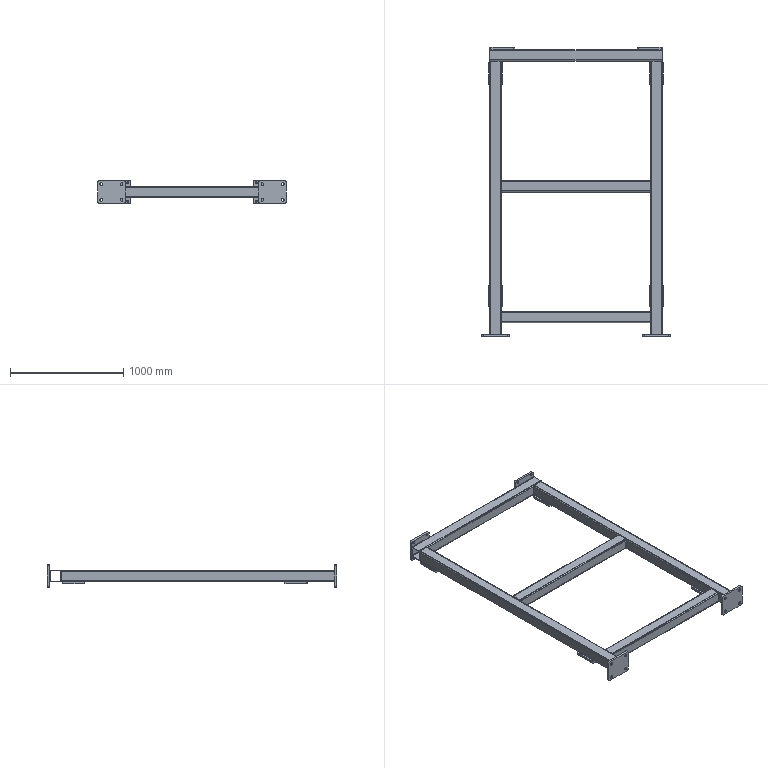Part | STEP file | 13 solids | 244 faces | box 1660 x 2550 x 200 mm | volume 21916544 mm3 | cylinder 126 | plane 118 | commonest cylinder face diameters 14 x38 20 x36 10 x20 18 x16 23 x16